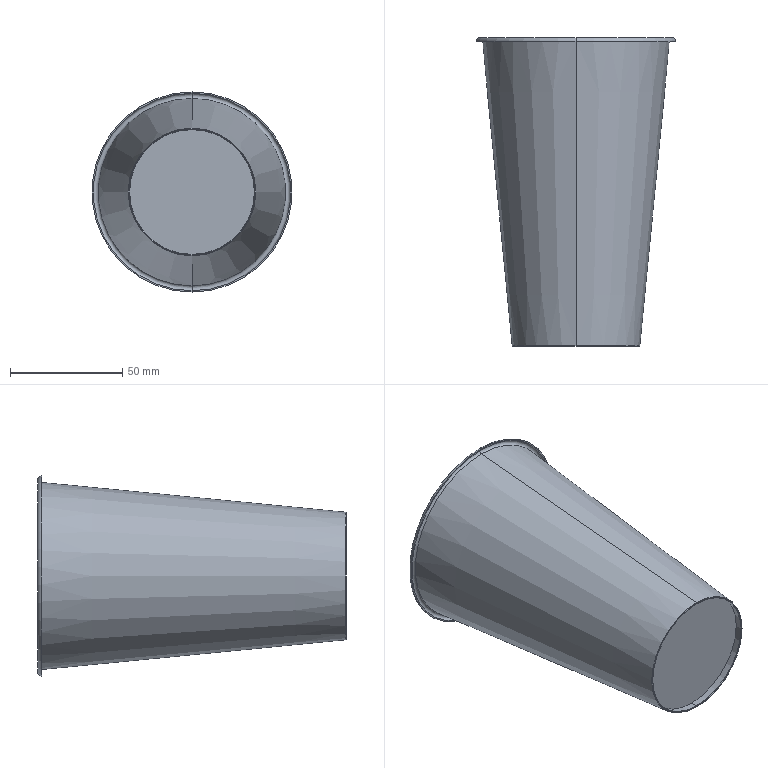Part | SolidWorks | features Revolution 1 | 1 solid | 20 faces | box 88.983 x 137.24 x 88.983 mm | volume 20015 mm3 | torus 10 | cone 6 | plane 4
STEP:
#1=CARTESIAN_POINT('',(0.,-3.86,-27.774));
#2=VERTEX_POINT('',#1);
#3=CARTESIAN_POINT('',(0.,-4.06,-27.974));
#4=VERTEX_POINT('',#3);
#5=CARTESIAN_POINT('',(0.,-3.86,-27.974));
#6=DIRECTION('',(1.,0.,0.));
#7=DIRECTION('',(0.,0.,-1.));
#8=AXIS2_PLACEMENT_3D('',#5,#6,#7);
#9=CIRCLE('',#8,0.2);
#10=EDGE_CURVE('',#2,#4,#9,.T.);
#11=ORIENTED_EDGE('',*,*,#10,.F.);
#12=CARTESIAN_POINT('',(0.,-3.86,27.774));
#13=VERTEX_POINT('',#12);
#14=CARTESIAN_POINT('',(0.,-3.86,0.));
#15=DIRECTION('',(0.,1.,0.));
#16=DIRECTION('',(0.,0.,1.));
#17=AXIS2_PLACEMENT_3D('',#14,#15,#16);
#18=CIRCLE('',#17,27.774);
#19=EDGE_CURVE('',#2,#13,#18,.T.);
#20=ORIENTED_EDGE('',*,*,#19,.T.);
#21=CARTESIAN_POINT('',(0.,-4.06,27.974));
#22=VERTEX_POINT('',#21);
#23=CARTESIAN_POINT('',(0.,-3.86,27.974));
#24=DIRECTION('',(-1.,0.,0.));
#25=DIRECTION('',(0.,0.,1.));
#26=AXIS2_PLACEMENT_3D('',#23,#24,#25);
#27=CIRCLE('',#26,0.2);
#28=EDGE_CURVE('',#13,#22,#27,.T.);
#29=ORIENTED_EDGE('',*,*,#28,.T.);
#30=CARTESIAN_POINT('',(0.,-4.06,0.));
#31=DIRECTION('',(0.,1.,0.));
#32=DIRECTION('',(0.,0.,1.));
#33=AXIS2_PLACEMENT_3D('',#30,#31,#32);
#34=CIRCLE('',#33,27.974);
#35=EDGE_CURVE('',#4,#22,#34,.T.);
#36=ORIENTED_EDGE('',*,*,#35,.F.);
#37=EDGE_LOOP('',(#11,#20,#29,#36));
#38=FACE_OUTER_BOUND('',#37,.T.);
#39=CARTESIAN_POINT('',(0.,-3.86,0.));
#40=DIRECTION('',(0.,1.,0.));
#41=DIRECTION('',(0.,0.,1.));
#42=AXIS2_PLACEMENT_3D('',#39,#40,#41);
#43=TOROIDAL_SURFACE('',#42,27.974,0.2);
#44=ADVANCED_FACE('',(#38),#43,.T.);
#45=ORIENTED_EDGE('',*,*,#28,.F.);
#46=CARTESIAN_POINT('',(0.,-3.86,0.));
#47=DIRECTION('',(0.,1.,0.));
#48=DIRECTION('',(0.,0.,1.));
#49=AXIS2_PLACEMENT_3D('',#46,#47,#48);
#50=CIRCLE('',#49,27.774);
#51=EDGE_CURVE('',#13,#2,#50,.T.);
#52=ORIENTED_EDGE('',*,*,#51,.T.);
#53=ORIENTED_EDGE('',*,*,#10,.T.);
#54=CARTESIAN_POINT('',(0.,-4.06,0.));
#55=DIRECTION('',(0.,1.,0.));
#56=DIRECTION('',(0.,0.,1.));
#57=AXIS2_PLACEMENT_3D('',#54,#55,#56);
#58=CIRCLE('',#57,27.974);
#59=EDGE_CURVE('',#22,#4,#58,.T.);
#60=ORIENTED_EDGE('',*,*,#59,.F.);
#61=EDGE_LOOP('',(#45,#52,#53,#60));
#62=FACE_OUTER_BOUND('',#61,.T.);
#63=CARTESIAN_POINT('',(0.,-3.86,0.));
#64=DIRECTION('',(0.,1.,0.));
#65=DIRECTION('',(0.,0.,1.));
#66=AXIS2_PLACEMENT_3D('',#63,#64,#65);
#67=TOROIDAL_SURFACE('',#66,27.974,0.2);
#68=ADVANCED_FACE('',(#62),#67,.T.);
#69=CARTESIAN_POINT('',(0.,-3.841,-27.775));
#70=VERTEX_POINT('',#69);
#71=CARTESIAN_POINT('',(0.,-3.841,27.775));
#72=VERTEX_POINT('',#71);
#73=CARTESIAN_POINT('',(0.,-3.841,0.));
#74=DIRECTION('',(0.,1.,0.));
#75=DIRECTION('',(0.,0.,1.));
#76=AXIS2_PLACEMENT_3D('',#73,#74,#75);
#77=CIRCLE('',#76,27.775);
#78=EDGE_CURVE('',#70,#72,#77,.T.);
#79=ORIENTED_EDGE('',*,*,#78,.F.);
#80=CARTESIAN_POINT('',(0.,-0.6,-28.091));
#81=VERTEX_POINT('',#80);
#82=CARTESIAN_POINT('',(0.,-0.6,-28.091));
#83=DIRECTION('',(0.,0.9953,-0.09718));
#84=VECTOR('',#83,1000.);
#85=LINE('',#82,#84);
#86=EDGE_CURVE('',#70,#81,#85,.T.);
#87=ORIENTED_EDGE('',*,*,#86,.T.);
#88=CARTESIAN_POINT('',(0.,-0.6,28.091));
#89=VERTEX_POINT('',#88);
#90=CARTESIAN_POINT('',(0.,-0.6,0.));
#91=DIRECTION('',(0.,1.,0.));
#92=DIRECTION('',(0.,0.,1.));
#93=AXIS2_PLACEMENT_3D('',#90,#91,#92);
#94=CIRCLE('',#93,28.091);
#95=EDGE_CURVE('',#81,#89,#94,.T.);
#96=ORIENTED_EDGE('',*,*,#95,.T.);
#97=CARTESIAN_POINT('',(0.,-0.6,28.091));
#98=DIRECTION('',(0.,0.9953,0.09718));
#99=VECTOR('',#98,1000.);
#100=LINE('',#97,#99);
#101=EDGE_CURVE('',#72,#89,#100,.T.);
#102=ORIENTED_EDGE('',*,*,#101,.F.);
#103=EDGE_LOOP('',(#79,#87,#96,#102));
#104=FACE_OUTER_BOUND('',#103,.T.);
#105=CARTESIAN_POINT('',(0.,-0.6,0.));
#106=DIRECTION('',(0.,1.,0.));
#107=DIRECTION('',(0.,0.,1.));
#108=AXIS2_PLACEMENT_3D('',#105,#106,#107);
#109=CONICAL_SURFACE('',#108,28.091,0.09734);
#110=ADVANCED_FACE('',(#104),#109,.F.);
#111=ORIENTED_EDGE('',*,*,#51,.F.);
#112=CARTESIAN_POINT('',(0.,-3.86,27.974));
#113=DIRECTION('',(-1.,0.,0.));
#114=DIRECTION('',(0.,0.,1.));
#115=AXIS2_PLACEMENT_3D('',#112,#113,#114);
#116=CIRCLE('',#115,0.2);
#117=EDGE_CURVE('',#72,#13,#116,.T.);
#118=ORIENTED_EDGE('',*,*,#117,.F.);
#119=CARTESIAN_POINT('',(0.,-3.841,0.));
#120=DIRECTION('',(0.,1.,0.));
#121=DIRECTION('',(0.,0.,1.));
#122=AXIS2_PLACEMENT_3D('',#119,#120,#121);
#123=CIRCLE('',#122,27.775);
#124=EDGE_CURVE('',#72,#70,#123,.T.);
#125=ORIENTED_EDGE('',*,*,#124,.T.);
#126=CARTESIAN_POINT('',(0.,-3.86,-27.974));
#127=DIRECTION('',(1.,0.,0.));
#128=DIRECTION('',(0.,0.,-1.));
#129=AXIS2_PLACEMENT_3D('',#126,#127,#128);
#130=CIRCLE('',#129,0.2);
#131=EDGE_CURVE('',#70,#2,#130,.T.);
#132=ORIENTED_EDGE('',*,*,#131,.T.);
#133=EDGE_LOOP('',(#111,#118,#125,#132));
#134=FACE_OUTER_BOUND('',#133,.T.);
#135=CARTESIAN_POINT('',(0.,-3.86,0.));
#136=DIRECTION('',(0.,1.,0.));
#137=DIRECTION('',(0.,0.,1.));
#138=AXIS2_PLACEMENT_3D('',#135,#136,#137);
#139=TOROIDAL_SURFACE('',#138,27.974,0.2);
#140=ADVANCED_FACE('',(#134),#139,.T.);
#141=CARTESIAN_POINT('',(0.,-4.06,28.175));
#142=VERTEX_POINT('',#141);
#143=CARTESIAN_POINT('',(0.,-4.06,-28.175));
#144=VERTEX_POINT('',#143);
#145=CARTESIAN_POINT('',(0.,-4.06,0.));
#146=DIRECTION('',(0.,1.,0.));
#147=DIRECTION('',(0.,0.,1.));
#148=AXIS2_PLACEMENT_3D('',#145,#146,#147);
#149=CIRCLE('',#148,28.175);
#150=EDGE_CURVE('',#142,#144,#149,.T.);
#151=ORIENTED_EDGE('',*,*,#150,.T.);
#152=CARTESIAN_POINT('',(0.,-3.879,-28.374));
#153=VERTEX_POINT('',#152);
#154=CARTESIAN_POINT('',(0.,-3.86,-28.175));
#155=DIRECTION('',(1.,0.,0.));
#156=DIRECTION('',(0.,0.,-1.));
#157=AXIS2_PLACEMENT_3D('',#154,#155,#156);
#158=CIRCLE('',#157,0.2);
#159=EDGE_CURVE('',#144,#153,#158,.T.);
#160=ORIENTED_EDGE('',*,*,#159,.T.);
#161=CARTESIAN_POINT('',(0.,-3.879,28.374));
#162=VERTEX_POINT('',#161);
#163=CARTESIAN_POINT('',(0.,-3.879,0.));
#164=DIRECTION('',(0.,1.,0.));
#165=DIRECTION('',(0.,0.,1.));
#166=AXIS2_PLACEMENT_3D('',#163,#164,#165);
#167=CIRCLE('',#166,28.374);
#168=EDGE_CURVE('',#162,#153,#167,.T.);
#169=ORIENTED_EDGE('',*,*,#168,.F.);
#170=CARTESIAN_POINT('',(0.,-3.86,28.175));
#171=DIRECTION('',(-1.,0.,0.));
#172=DIRECTION('',(0.,0.,1.));
#173=AXIS2_PLACEMENT_3D('',#170,#171,#172);
#174=CIRCLE('',#173,0.2);
#175=EDGE_CURVE('',#142,#162,#174,.T.);
#176=ORIENTED_EDGE('',*,*,#175,.F.);
#177=EDGE_LOOP('',(#151,#160,#169,#176));
#178=FACE_OUTER_BOUND('',#177,.T.);
#179=CARTESIAN_POINT('',(0.,-3.86,0.));
#180=DIRECTION('',(0.,1.,0.));
#181=DIRECTION('',(0.,0.,1.));
#182=AXIS2_PLACEMENT_3D('',#179,#180,#181);
#183=TOROIDAL_SURFACE('',#182,28.175,0.2);
#184=ADVANCED_FACE('',(#178),#183,.T.);
#185=ORIENTED_EDGE('',*,*,#168,.T.);
#186=CARTESIAN_POINT('',(0.,131.542,-41.597));
#187=VERTEX_POINT('',#186);
#188=CARTESIAN_POINT('',(0.,-3.879,-28.374));
#189=DIRECTION('',(0.,0.9953,-0.09718));
#190=VECTOR('',#189,1000.);
#191=LINE('',#188,#190);
#192=EDGE_CURVE('',#153,#187,#191,.T.);
#193=ORIENTED_EDGE('',*,*,#192,.T.);
#194=CARTESIAN_POINT('',(0.,131.542,41.597));
#195=VERTEX_POINT('',#194);
#196=CARTESIAN_POINT('',(0.,131.542,0.));
#197=DIRECTION('',(0.,1.,0.));
#198=DIRECTION('',(0.,0.,1.));
#199=AXIS2_PLACEMENT_3D('',#196,#197,#198);
#200=CIRCLE('',#199,41.597);
#201=EDGE_CURVE('',#195,#187,#200,.T.);
#202=ORIENTED_EDGE('',*,*,#201,.F.);
#203=CARTESIAN_POINT('',(0.,-3.879,28.374));
#204=DIRECTION('',(0.,0.9953,0.09718));
#205=VECTOR('',#204,1000.);
#206=LINE('',#203,#205);
#207=EDGE_CURVE('',#162,#195,#206,.T.);
#208=ORIENTED_EDGE('',*,*,#207,.F.);
#209=EDGE_LOOP('',(#185,#193,#202,#208));
#210=FACE_OUTER_BOUND('',#209,.T.);
#211=CARTESIAN_POINT('',(0.,-3.879,0.));
#212=DIRECTION('',(0.,1.,0.));
#213=DIRECTION('',(0.,0.,1.));
#214=AXIS2_PLACEMENT_3D('',#211,#212,#213);
#215=CONICAL_SURFACE('',#214,28.374,0.09734);
#216=ADVANCED_FACE('',(#210),#215,.T.);
#217=CARTESIAN_POINT('',(0.,131.43,-43.892));
#218=VERTEX_POINT('',#217);
#219=CARTESIAN_POINT('',(0.,131.43,43.892));
#220=VERTEX_POINT('',#219);
#221=CARTESIAN_POINT('',(0.,131.43,0.));
#222=DIRECTION('',(0.,1.,0.));
#223=DIRECTION('',(0.,0.,1.));
#224=AXIS2_PLACEMENT_3D('',#221,#222,#223);
#225=CIRCLE('',#224,43.892);
#226=EDGE_CURVE('',#218,#220,#225,.T.);
#227=ORIENTED_EDGE('',*,*,#226,.F.);
#228=CARTESIAN_POINT('',(0.,131.43,-42.742));
#229=DIRECTION('',(1.,0.,0.));
#230=DIRECTION('',(0.,0.,-1.));
#231=AXIS2_PLACEMENT_3D('',#228,#229,#230);
#232=CIRCLE('',#231,1.15);
#233=EDGE_CURVE('',#218,#187,#232,.T.);
#234=ORIENTED_EDGE('',*,*,#233,.T.);
#235=CARTESIAN_POINT('',(0.,131.542,0.));
#236=DIRECTION('',(0.,1.,0.));
#237=DIRECTION('',(0.,0.,1.));
#238=AXIS2_PLACEMENT_3D('',#235,#236,#237);
#239=CIRCLE('',#238,41.597);
#240=EDGE_CURVE('',#187,#195,#239,.T.);
#241=ORIENTED_EDGE('',*,*,#240,.T.);
#242=CARTESIAN_POINT('',(0.,131.43,42.742));
#243=DIRECTION('',(-1.,0.,0.));
#244=DIRECTION('',(0.,0.,1.));
#245=AXIS2_PLACEMENT_3D('',#242,#243,#244);
#246=CIRCLE('',#245,1.15);
#247=EDGE_CURVE('',#220,#195,#246,.T.);
#248=ORIENTED_EDGE('',*,*,#247,.F.);
#249=EDGE_LOOP('',(#227,#234,#241,#248));
#250=FACE_OUTER_BOUND('',#249,.T.);
#251=CARTESIAN_POINT('',(0.,131.43,0.));
#252=DIRECTION('',(0.,1.,0.));
#253=DIRECTION('',(0.,0.,1.));
#254=AXIS2_PLACEMENT_3D('',#251,#252,#253);
#255=TOROIDAL_SURFACE('',#254,42.742,1.15);
#256=ADVANCED_FACE('',(#250),#255,.F.);
#257=CARTESIAN_POINT('',(0.,131.43,44.492));
#258=VERTEX_POINT('',#257);
#259=CARTESIAN_POINT('',(0.,131.43,-44.492));
#260=VERTEX_POINT('',#259);
#261=CARTESIAN_POINT('',(0.,131.43,0.));
#262=DIRECTION('',(0.,1.,0.));
#263=DIRECTION('',(0.,0.,1.));
#264=AXIS2_PLACEMENT_3D('',#261,#262,#263);
#265=CIRCLE('',#264,44.492);
#266=EDGE_CURVE('',#258,#260,#265,.T.);
#267=ORIENTED_EDGE('',*,*,#266,.T.);
#268=CARTESIAN_POINT('',(0.,131.6,-41.));
#269=VERTEX_POINT('',#268);
#270=CARTESIAN_POINT('',(0.,131.43,-42.742));
#271=DIRECTION('',(1.,0.,0.));
#272=DIRECTION('',(0.,0.,-1.));
#273=AXIS2_PLACEMENT_3D('',#270,#271,#272);
#274=CIRCLE('',#273,1.75);
#275=EDGE_CURVE('',#260,#269,#274,.T.);
#276=ORIENTED_EDGE('',*,*,#275,.T.);
#277=CARTESIAN_POINT('',(0.,131.6,41.));
#278=VERTEX_POINT('',#277);
#279=CARTESIAN_POINT('',(0.,131.6,0.));
#280=DIRECTION('',(0.,1.,0.));
#281=DIRECTION('',(0.,0.,1.));
#282=AXIS2_PLACEMENT_3D('',#279,#280,#281);
#283=CIRCLE('',#282,41.);
#284=EDGE_CURVE('',#278,#269,#283,.T.);
#285=ORIENTED_EDGE('',*,*,#284,.F.);
#286=CARTESIAN_POINT('',(0.,131.43,42.742));
#287=DIRECTION('',(-1.,0.,0.));
#288=DIRECTION('',(0.,0.,1.));
#289=AXIS2_PLACEMENT_3D('',#286,#287,#288);
#290=CIRCLE('',#289,1.75);
#291=EDGE_CURVE('',#258,#278,#290,.T.);
#292=ORIENTED_EDGE('',*,*,#291,.F.);
#293=EDGE_LOOP('',(#267,#276,#285,#292));
#294=FACE_OUTER_BOUND('',#293,.T.);
#295=CARTESIAN_POINT('',(0.,131.43,0.));
#296=DIRECTION('',(0.,1.,0.));
#297=DIRECTION('',(0.,0.,1.));
#298=AXIS2_PLACEMENT_3D('',#295,#296,#297);
#299=TOROIDAL_SURFACE('',#298,42.742,1.75);
#300=ADVANCED_FACE('',(#294),#299,.T.);
#301=CARTESIAN_POINT('',(0.,0.,-28.15));
#302=VERTEX_POINT('',#301);
#303=CARTESIAN_POINT('',(0.,0.,28.15));
#304=VERTEX_POINT('',#303);
#305=CARTESIAN_POINT('',(0.,0.,0.));
#306=DIRECTION('',(0.,1.,0.));
#307=DIRECTION('',(0.,0.,1.));
#308=AXIS2_PLACEMENT_3D('',#305,#306,#307);
#309=CIRCLE('',#308,28.15);
#310=EDGE_CURVE('',#302,#304,#309,.T.);
#311=ORIENTED_EDGE('',*,*,#310,.F.);
#312=CARTESIAN_POINT('',(0.,131.6,-41.));
#313=DIRECTION('',(0.,0.9953,-0.09718));
#314=VECTOR('',#313,1000.);
#315=LINE('',#312,#314);
#316=EDGE_CURVE('',#302,#269,#315,.T.);
#317=ORIENTED_EDGE('',*,*,#316,.T.);
#318=CARTESIAN_POINT('',(0.,131.6,0.));
#319=DIRECTION('',(0.,1.,0.));
#320=DIRECTION('',(0.,0.,1.));
#321=AXIS2_PLACEMENT_3D('',#318,#319,#320);
#322=CIRCLE('',#321,41.);
#323=EDGE_CURVE('',#269,#278,#322,.T.);
#324=ORIENTED_EDGE('',*,*,#323,.T.);
#325=CARTESIAN_POINT('',(0.,131.6,41.));
#326=DIRECTION('',(0.,0.9953,0.09718));
#327=VECTOR('',#326,1000.);
#328=LINE('',#325,#327);
#329=EDGE_CURVE('',#304,#278,#328,.T.);
#330=ORIENTED_EDGE('',*,*,#329,.F.);
#331=EDGE_LOOP('',(#311,#317,#324,#330));
#332=FACE_OUTER_BOUND('',#331,.T.);
#333=CARTESIAN_POINT('',(0.,131.6,0.));
#334=DIRECTION('',(0.,1.,0.));
#335=DIRECTION('',(0.,0.,1.));
#336=AXIS2_PLACEMENT_3D('',#333,#334,#335);
#337=CONICAL_SURFACE('',#336,41.,0.09734);
#338=ADVANCED_FACE('',(#332),#337,.F.);
#339=CARTESIAN_POINT('',(0.,0.,0.));
#340=DIRECTION('',(0.,1.,0.));
#341=DIRECTION('',(0.,0.,1.));
#342=AXIS2_PLACEMENT_3D('',#339,#340,#341);
#343=CIRCLE('',#342,28.15);
#344=EDGE_CURVE('',#304,#302,#343,.T.);
#345=ORIENTED_EDGE('',*,*,#344,.T.);
#346=ORIENTED_EDGE('',*,*,#310,.T.);
#347=EDGE_LOOP('',(#345,#346));
#348=FACE_OUTER_BOUND('',#347,.T.);
#349=CARTESIAN_POINT('',(0.,0.,0.));
#350=DIRECTION('',(0.,-1.,0.));
#351=DIRECTION('',(0.,0.,-1.));
#352=AXIS2_PLACEMENT_3D('',#349,#350,#351);
#353=PLANE('',#352);
#354=ADVANCED_FACE('',(#348),#353,.F.);
#355=ORIENTED_EDGE('',*,*,#316,.F.);
#356=ORIENTED_EDGE('',*,*,#344,.F.);
#357=ORIENTED_EDGE('',*,*,#329,.T.);
#358=ORIENTED_EDGE('',*,*,#284,.T.);
#359=EDGE_LOOP('',(#355,#356,#357,#358));
#360=FACE_OUTER_BOUND('',#359,.T.);
#361=CARTESIAN_POINT('',(0.,131.6,0.));
#362=DIRECTION('',(0.,1.,0.));
#363=DIRECTION('',(0.,0.,1.));
#364=AXIS2_PLACEMENT_3D('',#361,#362,#363);
#365=CONICAL_SURFACE('',#364,41.,0.09734);
#366=ADVANCED_FACE('',(#360),#365,.F.);
#367=ORIENTED_EDGE('',*,*,#275,.F.);
#368=CARTESIAN_POINT('',(0.,131.43,0.));
#369=DIRECTION('',(0.,1.,0.));
#370=DIRECTION('',(0.,0.,1.));
#371=AXIS2_PLACEMENT_3D('',#368,#369,#370);
#372=CIRCLE('',#371,44.492);
#373=EDGE_CURVE('',#260,#258,#372,.T.);
#374=ORIENTED_EDGE('',*,*,#373,.T.);
#375=ORIENTED_EDGE('',*,*,#291,.T.);
#376=ORIENTED_EDGE('',*,*,#323,.F.);
#377=EDGE_LOOP('',(#367,#374,#375,#376));
#378=FACE_OUTER_BOUND('',#377,.T.);
#379=CARTESIAN_POINT('',(0.,131.43,0.));
#380=DIRECTION('',(0.,1.,0.));
#381=DIRECTION('',(0.,0.,1.));
#382=AXIS2_PLACEMENT_3D('',#379,#380,#381);
#383=TOROIDAL_SURFACE('',#382,42.742,1.75);
#384=ADVANCED_FACE('',(#378),#383,.T.);
#385=ORIENTED_EDGE('',*,*,#266,.F.);
#386=ORIENTED_EDGE('',*,*,#373,.F.);
#387=EDGE_LOOP('',(#385,#386));
#388=FACE_OUTER_BOUND('',#387,.T.);
#389=CARTESIAN_POINT('',(0.,131.43,0.));
#390=DIRECTION('',(0.,1.,0.));
#391=DIRECTION('',(0.,0.,1.));
#392=AXIS2_PLACEMENT_3D('',#389,#390,#391);
#393=CIRCLE('',#392,43.892);
#394=EDGE_CURVE('',#220,#218,#393,.T.);
#395=ORIENTED_EDGE('',*,*,#394,.T.);
#396=ORIENTED_EDGE('',*,*,#226,.T.);
#397=EDGE_LOOP('',(#395,#396));
#398=FACE_BOUND('',#397,.T.);
#399=CARTESIAN_POINT('',(43.892,131.43,0.));
#400=DIRECTION('',(0.,1.,0.));
#401=DIRECTION('',(0.,0.,1.));
#402=AXIS2_PLACEMENT_3D('',#399,#400,#401);
#403=PLANE('',#402);
#404=ADVANCED_FACE('',(#388,#398),#403,.F.);
#405=ORIENTED_EDGE('',*,*,#233,.F.);
#406=ORIENTED_EDGE('',*,*,#394,.F.);
#407=ORIENTED_EDGE('',*,*,#247,.T.);
#408=ORIENTED_EDGE('',*,*,#201,.T.);
#409=EDGE_LOOP('',(#405,#406,#407,#408));
#410=FACE_OUTER_BOUND('',#409,.T.);
#411=CARTESIAN_POINT('',(0.,131.43,0.));
#412=DIRECTION('',(0.,1.,0.));
#413=DIRECTION('',(0.,0.,1.));
#414=AXIS2_PLACEMENT_3D('',#411,#412,#413);
#415=TOROIDAL_SURFACE('',#414,42.742,1.15);
#416=ADVANCED_FACE('',(#410),#415,.F.);
#417=ORIENTED_EDGE('',*,*,#192,.F.);
#418=CARTESIAN_POINT('',(0.,-3.879,0.));
#419=DIRECTION('',(0.,1.,0.));
#420=DIRECTION('',(0.,0.,1.));
#421=AXIS2_PLACEMENT_3D('',#418,#419,#420);
#422=CIRCLE('',#421,28.374);
#423=EDGE_CURVE('',#153,#162,#422,.T.);
#424=ORIENTED_EDGE('',*,*,#423,.T.);
#425=ORIENTED_EDGE('',*,*,#207,.T.);
#426=ORIENTED_EDGE('',*,*,#240,.F.);
#427=EDGE_LOOP('',(#417,#424,#425,#426));
#428=FACE_OUTER_BOUND('',#427,.T.);
#429=CARTESIAN_POINT('',(0.,-3.879,0.));
#430=DIRECTION('',(0.,1.,0.));
#431=DIRECTION('',(0.,0.,1.));
#432=AXIS2_PLACEMENT_3D('',#429,#430,#431);
#433=CONICAL_SURFACE('',#432,28.374,0.09734);
#434=ADVANCED_FACE('',(#428),#433,.T.);
#435=ORIENTED_EDGE('',*,*,#159,.F.);
#436=CARTESIAN_POINT('',(0.,-4.06,0.));
#437=DIRECTION('',(0.,1.,0.));
#438=DIRECTION('',(0.,0.,1.));
#439=AXIS2_PLACEMENT_3D('',#436,#437,#438);
#440=CIRCLE('',#439,28.175);
#441=EDGE_CURVE('',#144,#142,#440,.T.);
#442=ORIENTED_EDGE('',*,*,#441,.T.);
#443=ORIENTED_EDGE('',*,*,#175,.T.);
#444=ORIENTED_EDGE('',*,*,#423,.F.);
#445=EDGE_LOOP('',(#435,#442,#443,#444));
#446=FACE_OUTER_BOUND('',#445,.T.);
#447=CARTESIAN_POINT('',(0.,-3.86,0.));
#448=DIRECTION('',(0.,1.,0.));
#449=DIRECTION('',(0.,0.,1.));
#450=AXIS2_PLACEMENT_3D('',#447,#448,#449);
#451=TOROIDAL_SURFACE('',#450,28.175,0.2);
#452=ADVANCED_FACE('',(#446),#451,.T.);
#453=ORIENTED_EDGE('',*,*,#150,.F.);
#454=ORIENTED_EDGE('',*,*,#441,.F.);
#455=EDGE_LOOP('',(#453,#454));
#456=FACE_OUTER_BOUND('',#455,.T.);
#457=ORIENTED_EDGE('',*,*,#59,.T.);
#458=ORIENTED_EDGE('',*,*,#35,.T.);
#459=EDGE_LOOP('',(#457,#458));
#460=FACE_BOUND('',#459,.T.);
#461=CARTESIAN_POINT('',(27.974,-4.06,0.));
#462=DIRECTION('',(0.,1.,0.));
#463=DIRECTION('',(0.,0.,1.));
#464=AXIS2_PLACEMENT_3D('',#461,#462,#463);
#465=PLANE('',#464);
#466=ADVANCED_FACE('',(#456,#460),#465,.F.);
#467=ORIENTED_EDGE('',*,*,#19,.F.);
#468=ORIENTED_EDGE('',*,*,#131,.F.);
#469=ORIENTED_EDGE('',*,*,#78,.T.);
#470=ORIENTED_EDGE('',*,*,#117,.T.);
#471=EDGE_LOOP('',(#467,#468,#469,#470));
#472=FACE_OUTER_BOUND('',#471,.T.);
#473=CARTESIAN_POINT('',(0.,-3.86,0.));
#474=DIRECTION('',(0.,1.,0.));
#475=DIRECTION('',(0.,0.,1.));
#476=AXIS2_PLACEMENT_3D('',#473,#474,#475);
#477=TOROIDAL_SURFACE('',#476,27.974,0.2);
#478=ADVANCED_FACE('',(#472),#477,.T.);
#479=ORIENTED_EDGE('',*,*,#86,.F.);
#480=ORIENTED_EDGE('',*,*,#124,.F.);
#481=ORIENTED_EDGE('',*,*,#101,.T.);
#482=CARTESIAN_POINT('',(0.,-0.6,0.));
#483=DIRECTION('',(0.,1.,0.));
#484=DIRECTION('',(0.,0.,1.));
#485=AXIS2_PLACEMENT_3D('',#482,#483,#484);
#486=CIRCLE('',#485,28.091);
#487=EDGE_CURVE('',#89,#81,#486,.T.);
#488=ORIENTED_EDGE('',*,*,#487,.T.);
#489=EDGE_LOOP('',(#479,#480,#481,#488));
#490=FACE_OUTER_BOUND('',#489,.T.);
#491=CARTESIAN_POINT('',(0.,-0.6,0.));
#492=DIRECTION('',(0.,1.,0.));
#493=DIRECTION('',(0.,0.,1.));
#494=AXIS2_PLACEMENT_3D('',#491,#492,#493);
#495=CONICAL_SURFACE('',#494,28.091,0.09734);
#496=ADVANCED_FACE('',(#490),#495,.F.);
#497=ORIENTED_EDGE('',*,*,#487,.F.);
#498=ORIENTED_EDGE('',*,*,#95,.F.);
#499=EDGE_LOOP('',(#497,#498));
#500=FACE_OUTER_BOUND('',#499,.T.);
#501=CARTESIAN_POINT('',(0.,-0.6,0.));
#502=DIRECTION('',(0.,1.,0.));
#503=DIRECTION('',(0.,0.,1.));
#504=AXIS2_PLACEMENT_3D('',#501,#502,#503);
#505=PLANE('',#504);
#506=ADVANCED_FACE('',(#500),#505,.F.);
#507=CLOSED_SHELL('',(#44,#68,#110,#140,#184,#216,#256,#300,#338,#354,#366,#384,#404,#416,#434,#452,#466,#478,#496,#506));
#508=MANIFOLD_SOLID_BREP('',#507);
#509=CARTESIAN_POINT('',(0.,0.,0.));
#510=DIRECTION('',(0.,0.,1.));
#511=DIRECTION('',(1.,0.,0.));
#512=AXIS2_PLACEMENT_3D('',#509,#510,#511);
#513=(LENGTH_UNIT()NAMED_UNIT(*)SI_UNIT(.MILLI.,.METRE.));
#514=UNCERTAINTY_MEASURE_WITH_UNIT(LENGTH_MEASURE(0.00001),#513,'','');
#515=(NAMED_UNIT(*)PLANE_ANGLE_UNIT()SI_UNIT($,.RADIAN.));
#516=(NAMED_UNIT(*)SI_UNIT($,.STERADIAN.)SOLID_ANGLE_UNIT());
#517=(GEOMETRIC_REPRESENTATION_CONTEXT(3)GLOBAL_UNCERTAINTY_ASSIGNED_CONTEXT((#514))GLOBAL_UNIT_ASSIGNED_CONTEXT((#513,#515,#516))REPRESENTATION_CONTEXT('',''));
#518=ADVANCED_BREP_SHAPE_REPRESENTATION('',(#508,#512),#517);